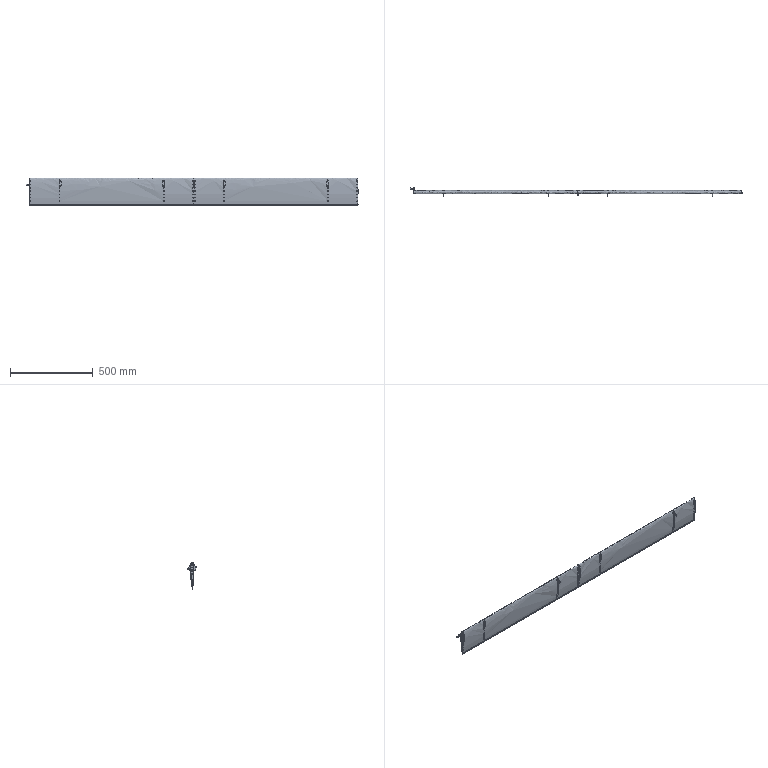Part | SolidWorks | features BaseBody 40 | 40 solids | 1151 faces | box 2003 x 52.2 x 165.107 mm | volume 656041 mm3 | cylinder 672 | plane 313 | spline 148 | cone 18 | commonest cylinder face diameters 3.2 x514 5 x48 3 x32 12 x28 2.614 x16 2.827 x8